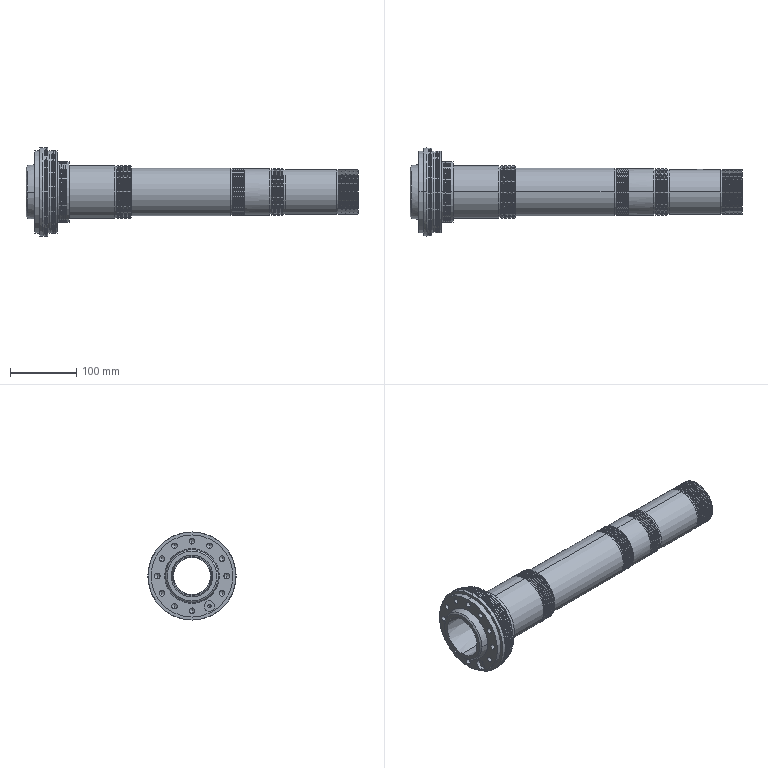Part | STEP file | 46 Spindle Inner Shaft | 1 solid | 381 faces | box 501 x 133 x 133 mm | volume 1064151 mm3 | cone 260 | cylinder 82 | plane 39 | commonest cylinder face diameters 8.5 x22 92 x10 124 x10 133 x6 8 x4 70 x4